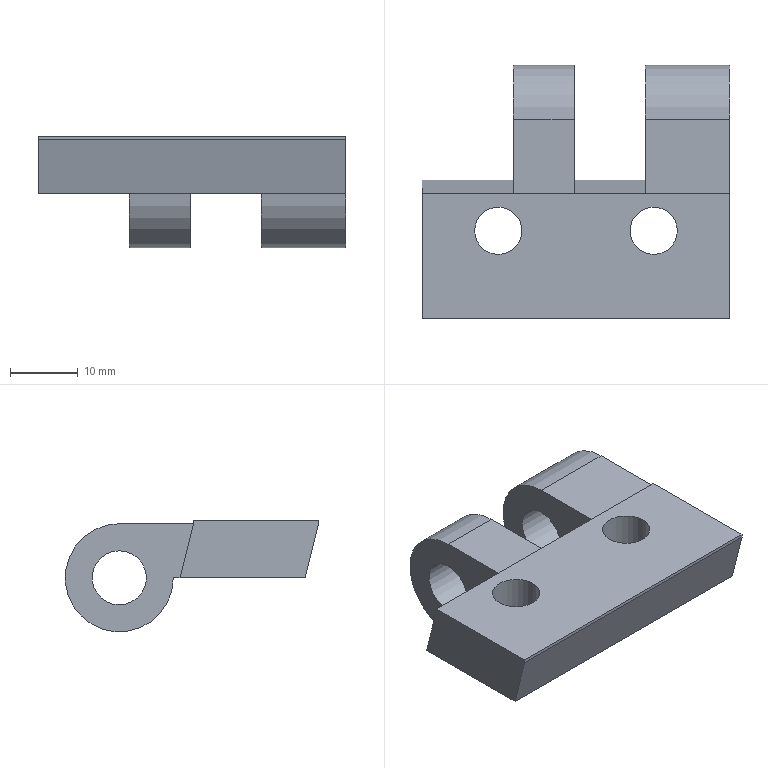Part | NX | 1 solid | 22 faces | box 45.5 x 37.5 x 16.5 mm | volume 10172 mm3 | plane 14 | cylinder 6 | cone 2 | commonest cylinder face diameters 7 x2 8 x2 16 x2
STEP:
#1=CARTESIAN_POINT('',(5.5,-8.5,-8.));
#2=VERTEX_POINT('',#1);
#3=CARTESIAN_POINT('',(11.75,-8.5,-8.));
#4=DIRECTION('',(0.,0.,-1.));
#5=DIRECTION('',(-1.,0.,0.));
#6=AXIS2_PLACEMENT_3D('',#3,#4,#5);
#7=CIRCLE('',#6,6.25);
#8=EDGE_CURVE('',#2,#2,#7,.T.);
#9=ORIENTED_EDGE('',*,*,#8,.F.);
#10=EDGE_LOOP('',(#9));
#11=FACE_BOUND('',#10,.T.);
#12=CARTESIAN_POINT('',(10.5,-1.,-8.));
#13=VERTEX_POINT('',#12);
#14=CARTESIAN_POINT('',(0.,-1.,-8.));
#15=VERTEX_POINT('',#14);
#16=CARTESIAN_POINT('',(10.5,-1.,-8.));
#17=DIRECTION('',(-1.,0.,0.));
#18=VECTOR('',#17,1000.);
#19=LINE('',#16,#18);
#20=EDGE_CURVE('',#13,#15,#19,.T.);
#21=ORIENTED_EDGE('',*,*,#20,.F.);
#22=CARTESIAN_POINT('',(10.5,0.,-8.));
#23=VERTEX_POINT('',#22);
#24=CARTESIAN_POINT('',(10.5,-1.,-8.));
#25=DIRECTION('',(0.,1.,0.));
#26=VECTOR('',#25,1000.);
#27=LINE('',#24,#26);
#28=EDGE_CURVE('',#13,#23,#27,.T.);
#29=ORIENTED_EDGE('',*,*,#28,.T.);
#30=CARTESIAN_POINT('',(23.,0.,-8.));
#31=VERTEX_POINT('',#30);
#32=CARTESIAN_POINT('',(10.5,0.,-8.));
#33=DIRECTION('',(1.,0.,0.));
#34=VECTOR('',#33,1000.);
#35=LINE('',#32,#34);
#36=EDGE_CURVE('',#23,#31,#35,.T.);
#37=ORIENTED_EDGE('',*,*,#36,.T.);
#38=CARTESIAN_POINT('',(23.,-19.5,-8.));
#39=VERTEX_POINT('',#38);
#40=CARTESIAN_POINT('',(23.,-21.5,-8.));
#41=DIRECTION('',(0.,1.,0.));
#42=VECTOR('',#41,1000.);
#43=LINE('',#40,#42);
#44=EDGE_CURVE('',#39,#31,#43,.T.);
#45=ORIENTED_EDGE('',*,*,#44,.F.);
#46=CARTESIAN_POINT('',(-22.5,-19.5,-8.));
#47=VERTEX_POINT('',#46);
#48=CARTESIAN_POINT('',(0.,-19.5,-8.));
#49=DIRECTION('',(-1.,0.,0.));
#50=VECTOR('',#49,1000.);
#51=LINE('',#48,#50);
#52=EDGE_CURVE('',#47,#39,#51,.F.);
#53=ORIENTED_EDGE('',*,*,#52,.F.);
#54=CARTESIAN_POINT('',(-22.5,-1.,-8.));
#55=VERTEX_POINT('',#54);
#56=CARTESIAN_POINT('',(-22.5,-21.5,-8.));
#57=DIRECTION('',(0.,-1.,0.));
#58=VECTOR('',#57,1000.);
#59=LINE('',#56,#58);
#60=EDGE_CURVE('',#55,#47,#59,.T.);
#61=ORIENTED_EDGE('',*,*,#60,.F.);
#62=CARTESIAN_POINT('',(-9.,-1.,-8.));
#63=VERTEX_POINT('',#62);
#64=CARTESIAN_POINT('',(-22.5,-1.,-8.));
#65=DIRECTION('',(1.,0.,0.));
#66=VECTOR('',#65,1000.);
#67=LINE('',#64,#66);
#68=EDGE_CURVE('',#55,#63,#67,.T.);
#69=ORIENTED_EDGE('',*,*,#68,.T.);
#70=CARTESIAN_POINT('',(-9.,0.,-8.));
#71=VERTEX_POINT('',#70);
#72=CARTESIAN_POINT('',(-9.,-21.5,-8.));
#73=DIRECTION('',(0.,-1.,0.));
#74=VECTOR('',#73,1000.);
#75=LINE('',#72,#74);
#76=EDGE_CURVE('',#71,#63,#75,.T.);
#77=ORIENTED_EDGE('',*,*,#76,.F.);
#78=CARTESIAN_POINT('',(0.,0.,-8.));
#79=VERTEX_POINT('',#78);
#80=CARTESIAN_POINT('',(-9.,0.,-8.));
#81=DIRECTION('',(1.,0.,0.));
#82=VECTOR('',#81,1000.);
#83=LINE('',#80,#82);
#84=EDGE_CURVE('',#71,#79,#83,.T.);
#85=ORIENTED_EDGE('',*,*,#84,.T.);
#86=CARTESIAN_POINT('',(0.,-21.5,-8.));
#87=DIRECTION('',(0.,-1.,0.));
#88=VECTOR('',#87,1000.);
#89=LINE('',#86,#88);
#90=EDGE_CURVE('',#79,#15,#89,.T.);
#91=ORIENTED_EDGE('',*,*,#90,.T.);
#92=EDGE_LOOP('',(#21,#29,#37,#45,#53,#61,#69,#77,#85,#91));
#93=FACE_BOUND('',#92,.T.);
#94=CARTESIAN_POINT('',(-17.5,-8.5,-8.));
#95=VERTEX_POINT('',#94);
#96=CARTESIAN_POINT('',(-11.25,-8.5,-8.));
#97=DIRECTION('',(0.,0.,-1.));
#98=DIRECTION('',(-1.,0.,0.));
#99=AXIS2_PLACEMENT_3D('',#96,#97,#98);
#100=CIRCLE('',#99,6.25);
#101=EDGE_CURVE('',#95,#95,#100,.T.);
#102=ORIENTED_EDGE('',*,*,#101,.F.);
#103=EDGE_LOOP('',(#102));
#104=FACE_BOUND('',#103,.T.);
#105=CARTESIAN_POINT('',(23.,-21.5,-8.));
#106=DIRECTION('',(0.,0.,1.));
#107=DIRECTION('',(1.,0.,0.));
#108=AXIS2_PLACEMENT_3D('',#105,#106,#107);
#109=PLANE('',#108);
#110=ADVANCED_FACE('',(#11,#93,#104),#109,.F.);
#111=CARTESIAN_POINT('',(-9.,-3.,0.));
#112=VERTEX_POINT('',#111);
#113=CARTESIAN_POINT('',(-9.,8.,0.));
#114=VERTEX_POINT('',#113);
#115=CARTESIAN_POINT('',(-9.,8.,0.));
#116=DIRECTION('',(0.,1.,0.));
#117=VECTOR('',#116,1000.);
#118=LINE('',#115,#117);
#119=EDGE_CURVE('',#112,#114,#118,.T.);
#120=ORIENTED_EDGE('',*,*,#119,.F.);
#121=CARTESIAN_POINT('',(0.,-3.,0.));
#122=VERTEX_POINT('',#121);
#123=CARTESIAN_POINT('',(-22.5,-3.,0.));
#124=DIRECTION('',(-1.,0.,0.));
#125=VECTOR('',#124,1000.);
#126=LINE('',#123,#125);
#127=EDGE_CURVE('',#122,#112,#126,.T.);
#128=ORIENTED_EDGE('',*,*,#127,.F.);
#129=CARTESIAN_POINT('',(0.,8.,0.));
#130=VERTEX_POINT('',#129);
#131=CARTESIAN_POINT('',(0.,8.,0.));
#132=DIRECTION('',(0.,1.,0.));
#133=VECTOR('',#132,1000.);
#134=LINE('',#131,#133);
#135=EDGE_CURVE('',#122,#130,#134,.T.);
#136=ORIENTED_EDGE('',*,*,#135,.T.);
#137=CARTESIAN_POINT('',(-9.,8.,0.));
#138=DIRECTION('',(1.,0.,0.));
#139=VECTOR('',#138,1000.);
#140=LINE('',#137,#139);
#141=EDGE_CURVE('',#114,#130,#140,.T.);
#142=ORIENTED_EDGE('',*,*,#141,.F.);
#143=EDGE_LOOP('',(#120,#128,#136,#142));
#144=FACE_BOUND('',#143,.T.);
#145=CARTESIAN_POINT('',(10.5,8.,0.));
#146=DIRECTION('',(0.,0.,1.));
#147=DIRECTION('',(1.,0.,0.));
#148=AXIS2_PLACEMENT_3D('',#145,#146,#147);
#149=PLANE('',#148);
#150=ADVANCED_FACE('',(#144),#149,.T.);
#151=CARTESIAN_POINT('',(10.5,8.,0.));
#152=VERTEX_POINT('',#151);
#153=CARTESIAN_POINT('',(10.5,-3.,0.));
#154=VERTEX_POINT('',#153);
#155=CARTESIAN_POINT('',(10.5,8.,0.));
#156=DIRECTION('',(0.,-1.,0.));
#157=VECTOR('',#156,1000.);
#158=LINE('',#155,#157);
#159=EDGE_CURVE('',#152,#154,#158,.T.);
#160=ORIENTED_EDGE('',*,*,#159,.T.);
#161=CARTESIAN_POINT('',(23.,-3.,0.));
#162=VERTEX_POINT('',#161);
#163=CARTESIAN_POINT('',(-22.5,-3.,0.));
#164=DIRECTION('',(-1.,0.,0.));
#165=VECTOR('',#164,1000.);
#166=LINE('',#163,#165);
#167=EDGE_CURVE('',#162,#154,#166,.T.);
#168=ORIENTED_EDGE('',*,*,#167,.F.);
#169=CARTESIAN_POINT('',(23.,8.,0.));
#170=VERTEX_POINT('',#169);
#171=CARTESIAN_POINT('',(23.,8.,0.));
#172=DIRECTION('',(0.,-1.,0.));
#173=VECTOR('',#172,1000.);
#174=LINE('',#171,#173);
#175=EDGE_CURVE('',#170,#162,#174,.T.);
#176=ORIENTED_EDGE('',*,*,#175,.F.);
#177=CARTESIAN_POINT('',(10.5,8.,0.));
#178=DIRECTION('',(1.,0.,0.));
#179=VECTOR('',#178,1000.);
#180=LINE('',#177,#179);
#181=EDGE_CURVE('',#152,#170,#180,.T.);
#182=ORIENTED_EDGE('',*,*,#181,.F.);
#183=EDGE_LOOP('',(#160,#168,#176,#182));
#184=FACE_BOUND('',#183,.T.);
#185=CARTESIAN_POINT('',(10.5,8.,0.));
#186=DIRECTION('',(0.,0.,1.));
#187=DIRECTION('',(1.,0.,0.));
#188=AXIS2_PLACEMENT_3D('',#185,#186,#187);
#189=PLANE('',#188);
#190=ADVANCED_FACE('',(#184),#189,.T.);
#191=CARTESIAN_POINT('',(-9.,8.,-12.));
#192=VERTEX_POINT('',#191);
#193=CARTESIAN_POINT('',(-9.,8.,-8.));
#194=DIRECTION('',(1.,0.,0.));
#195=DIRECTION('',(0.,0.,-1.));
#196=AXIS2_PLACEMENT_3D('',#193,#194,#195);
#197=CIRCLE('',#196,4.);
#198=EDGE_CURVE('',#192,#192,#197,.T.);
#199=ORIENTED_EDGE('',*,*,#198,.T.);
#200=EDGE_LOOP('',(#199));
#201=FACE_BOUND('',#200,.T.);
#202=CARTESIAN_POINT('',(-9.,-0.4706,-10.118));
#203=DIRECTION('',(0.,-0.2425,0.9701));
#204=VECTOR('',#203,1000.);
#205=LINE('',#202,#204);
#206=EDGE_CURVE('',#112,#63,#205,.F.);
#207=ORIENTED_EDGE('',*,*,#206,.F.);
#208=ORIENTED_EDGE('',*,*,#119,.T.);
#209=CARTESIAN_POINT('',(-9.,8.,-8.));
#210=DIRECTION('',(-1.,0.,0.));
#211=DIRECTION('',(0.,0.,-1.));
#212=AXIS2_PLACEMENT_3D('',#209,#210,#211);
#213=CIRCLE('',#212,8.);
#214=EDGE_CURVE('',#114,#71,#213,.T.);
#215=ORIENTED_EDGE('',*,*,#214,.T.);
#216=ORIENTED_EDGE('',*,*,#76,.T.);
#217=EDGE_LOOP('',(#207,#208,#215,#216));
#218=FACE_BOUND('',#217,.T.);
#219=CARTESIAN_POINT('',(-9.,8.,-8.));
#220=DIRECTION('',(1.,0.,0.));
#221=DIRECTION('',(0.,0.,-1.));
#222=AXIS2_PLACEMENT_3D('',#219,#220,#221);
#223=PLANE('',#222);
#224=ADVANCED_FACE('',(#201,#218),#223,.F.);
#225=CARTESIAN_POINT('',(23.,8.,-8.));
#226=DIRECTION('',(1.,0.,0.));
#227=DIRECTION('',(0.,0.,-1.));
#228=AXIS2_PLACEMENT_3D('',#225,#226,#227);
#229=CIRCLE('',#228,8.);
#230=EDGE_CURVE('',#31,#170,#229,.T.);
#231=ORIENTED_EDGE('',*,*,#230,.F.);
#232=ORIENTED_EDGE('',*,*,#36,.F.);
#233=CARTESIAN_POINT('',(10.5,8.,-8.));
#234=DIRECTION('',(1.,0.,0.));
#235=DIRECTION('',(0.,0.,-1.));
#236=AXIS2_PLACEMENT_3D('',#233,#234,#235);
#237=CIRCLE('',#236,8.);
#238=EDGE_CURVE('',#23,#152,#237,.T.);
#239=ORIENTED_EDGE('',*,*,#238,.T.);
#240=ORIENTED_EDGE('',*,*,#181,.T.);
#241=EDGE_LOOP('',(#231,#232,#239,#240));
#242=FACE_BOUND('',#241,.T.);
#243=CARTESIAN_POINT('',(10.5,8.,-8.));
#244=DIRECTION('',(1.,0.,0.));
#245=DIRECTION('',(0.,0.,-1.));
#246=AXIS2_PLACEMENT_3D('',#243,#244,#245);
#247=CYLINDRICAL_SURFACE('',#246,8.);
#248=ADVANCED_FACE('',(#242),#247,.T.);
#249=CARTESIAN_POINT('',(10.5,8.,-12.));
#250=VERTEX_POINT('',#249);
#251=CARTESIAN_POINT('',(10.5,8.,-8.));
#252=DIRECTION('',(1.,0.,0.));
#253=DIRECTION('',(0.,0.,-1.));
#254=AXIS2_PLACEMENT_3D('',#251,#252,#253);
#255=CIRCLE('',#254,4.);
#256=EDGE_CURVE('',#250,#250,#255,.T.);
#257=ORIENTED_EDGE('',*,*,#256,.T.);
#258=EDGE_LOOP('',(#257));
#259=FACE_BOUND('',#258,.T.);
#260=ORIENTED_EDGE('',*,*,#238,.F.);
#261=ORIENTED_EDGE('',*,*,#28,.F.);
#262=CARTESIAN_POINT('',(10.5,-1.,-8.));
#263=DIRECTION('',(0.,0.2425,-0.9701));
#264=VECTOR('',#263,1000.);
#265=LINE('',#262,#264);
#266=EDGE_CURVE('',#154,#13,#265,.T.);
#267=ORIENTED_EDGE('',*,*,#266,.F.);
#268=ORIENTED_EDGE('',*,*,#159,.F.);
#269=EDGE_LOOP('',(#260,#261,#267,#268));
#270=FACE_BOUND('',#269,.T.);
#271=CARTESIAN_POINT('',(10.5,8.,-8.));
#272=DIRECTION('',(1.,0.,0.));
#273=DIRECTION('',(0.,0.,-1.));
#274=AXIS2_PLACEMENT_3D('',#271,#272,#273);
#275=PLANE('',#274);
#276=ADVANCED_FACE('',(#259,#270),#275,.F.);
#277=CARTESIAN_POINT('',(23.,8.,-12.));
#278=VERTEX_POINT('',#277);
#279=CARTESIAN_POINT('',(23.,8.,-8.));
#280=DIRECTION('',(1.,0.,0.));
#281=DIRECTION('',(0.,0.,-1.));
#282=AXIS2_PLACEMENT_3D('',#279,#280,#281);
#283=CIRCLE('',#282,4.);
#284=EDGE_CURVE('',#278,#278,#283,.T.);
#285=ORIENTED_EDGE('',*,*,#284,.F.);
#286=EDGE_LOOP('',(#285));
#287=FACE_BOUND('',#286,.T.);
#288=ORIENTED_EDGE('',*,*,#230,.T.);
#289=ORIENTED_EDGE('',*,*,#175,.T.);
#290=CARTESIAN_POINT('',(23.,-3.,0.5));
#291=VERTEX_POINT('',#290);
#292=CARTESIAN_POINT('',(23.,-3.,0.5));
#293=DIRECTION('',(0.,0.,-1.));
#294=VECTOR('',#293,1000.);
#295=LINE('',#292,#294);
#296=EDGE_CURVE('',#291,#162,#295,.T.);
#297=ORIENTED_EDGE('',*,*,#296,.F.);
#298=CARTESIAN_POINT('',(23.,-21.5,0.5));
#299=VERTEX_POINT('',#298);
#300=CARTESIAN_POINT('',(23.,-3.,0.5));
#301=DIRECTION('',(0.,1.,0.));
#302=VECTOR('',#301,1000.);
#303=LINE('',#300,#302);
#304=EDGE_CURVE('',#299,#291,#303,.T.);
#305=ORIENTED_EDGE('',*,*,#304,.F.);
#306=CARTESIAN_POINT('',(23.,-21.5,0.));
#307=VERTEX_POINT('',#306);
#308=CARTESIAN_POINT('',(23.,-21.5,0.5));
#309=DIRECTION('',(0.,0.,-1.));
#310=VECTOR('',#309,1000.);
#311=LINE('',#308,#310);
#312=EDGE_CURVE('',#299,#307,#311,.T.);
#313=ORIENTED_EDGE('',*,*,#312,.T.);
#314=CARTESIAN_POINT('',(23.,-17.882,-14.471));
#315=DIRECTION('',(0.,0.2425,-0.9701));
#316=VECTOR('',#315,1000.);
#317=LINE('',#314,#316);
#318=EDGE_CURVE('',#39,#307,#317,.F.);
#319=ORIENTED_EDGE('',*,*,#318,.F.);
#320=ORIENTED_EDGE('',*,*,#44,.T.);
#321=EDGE_LOOP('',(#288,#289,#297,#305,#313,#319,#320));
#322=FACE_BOUND('',#321,.T.);
#323=CARTESIAN_POINT('',(23.,8.,-8.));
#324=DIRECTION('',(1.,0.,0.));
#325=DIRECTION('',(0.,0.,-1.));
#326=AXIS2_PLACEMENT_3D('',#323,#324,#325);
#327=PLANE('',#326);
#328=ADVANCED_FACE('',(#287,#322),#327,.T.);
#329=CARTESIAN_POINT('',(-22.5,-21.5,0.));
#330=VERTEX_POINT('',#329);
#331=CARTESIAN_POINT('',(0.,-21.5,0.));
#332=DIRECTION('',(-1.,0.,0.));
#333=VECTOR('',#332,1000.);
#334=LINE('',#331,#333);
#335=EDGE_CURVE('',#307,#330,#334,.T.);
#336=ORIENTED_EDGE('',*,*,#335,.T.);
#337=CARTESIAN_POINT('',(-22.5,-20.235,-5.059));
#338=DIRECTION('',(0.,0.2425,-0.9701));
#339=VECTOR('',#338,1000.);
#340=LINE('',#337,#339);
#341=EDGE_CURVE('',#47,#330,#340,.F.);
#342=ORIENTED_EDGE('',*,*,#341,.F.);
#343=ORIENTED_EDGE('',*,*,#52,.T.);
#344=ORIENTED_EDGE('',*,*,#318,.T.);
#345=EDGE_LOOP('',(#336,#342,#343,#344));
#346=FACE_BOUND('',#345,.T.);
#347=CARTESIAN_POINT('',(0.,-21.5,0.));
#348=DIRECTION('',(0.,-0.9701,-0.2425));
#349=DIRECTION('',(0.,0.2425,-0.9701));
#350=AXIS2_PLACEMENT_3D('',#347,#348,#349);
#351=PLANE('',#350);
#352=ADVANCED_FACE('',(#346),#351,.T.);
#353=ORIENTED_EDGE('',*,*,#266,.T.);
#354=ORIENTED_EDGE('',*,*,#20,.T.);
#355=CARTESIAN_POINT('',(0.,-0.4706,-10.118));
#356=DIRECTION('',(0.,-0.2425,0.9701));
#357=VECTOR('',#356,1000.);
#358=LINE('',#355,#357);
#359=EDGE_CURVE('',#15,#122,#358,.T.);
#360=ORIENTED_EDGE('',*,*,#359,.T.);
#361=CARTESIAN_POINT('',(10.5,-3.,0.));
#362=DIRECTION('',(1.,0.,0.));
#363=VECTOR('',#362,1000.);
#364=LINE('',#361,#363);
#365=EDGE_CURVE('',#122,#154,#364,.T.);
#366=ORIENTED_EDGE('',*,*,#365,.T.);
#367=EDGE_LOOP('',(#353,#354,#360,#366));
#368=FACE_BOUND('',#367,.T.);
#369=CARTESIAN_POINT('',(10.5,-1.,-8.));
#370=DIRECTION('',(0.,0.9701,0.2425));
#371=DIRECTION('',(0.,-0.2425,0.9701));
#372=AXIS2_PLACEMENT_3D('',#369,#370,#371);
#373=PLANE('',#372);
#374=ADVANCED_FACE('',(#368),#373,.T.);
#375=CARTESIAN_POINT('',(0.,8.,-12.));
#376=VERTEX_POINT('',#375);
#377=CARTESIAN_POINT('',(0.,8.,-8.));
#378=DIRECTION('',(1.,0.,0.));
#379=DIRECTION('',(0.,0.,-1.));
#380=AXIS2_PLACEMENT_3D('',#377,#378,#379);
#381=CIRCLE('',#380,4.);
#382=EDGE_CURVE('',#376,#376,#381,.T.);
#383=ORIENTED_EDGE('',*,*,#382,.F.);
#384=EDGE_LOOP('',(#383));
#385=FACE_BOUND('',#384,.T.);
#386=ORIENTED_EDGE('',*,*,#359,.F.);
#387=ORIENTED_EDGE('',*,*,#90,.F.);
#388=CARTESIAN_POINT('',(0.,8.,-8.));
#389=DIRECTION('',(-1.,0.,0.));
#390=DIRECTION('',(0.,0.,-1.));
#391=AXIS2_PLACEMENT_3D('',#388,#389,#390);
#392=CIRCLE('',#391,8.);
#393=EDGE_CURVE('',#130,#79,#392,.T.);
#394=ORIENTED_EDGE('',*,*,#393,.F.);
#395=ORIENTED_EDGE('',*,*,#135,.F.);
#396=EDGE_LOOP('',(#386,#387,#394,#395));
#397=FACE_BOUND('',#396,.T.);
#398=CARTESIAN_POINT('',(0.,8.,-8.));
#399=DIRECTION('',(1.,0.,0.));
#400=DIRECTION('',(0.,0.,-1.));
#401=AXIS2_PLACEMENT_3D('',#398,#399,#400);
#402=PLANE('',#401);
#403=ADVANCED_FACE('',(#385,#397),#402,.T.);
#404=ORIENTED_EDGE('',*,*,#393,.T.);
#405=ORIENTED_EDGE('',*,*,#84,.F.);
#406=ORIENTED_EDGE('',*,*,#214,.F.);
#407=ORIENTED_EDGE('',*,*,#141,.T.);
#408=EDGE_LOOP('',(#404,#405,#406,#407));
#409=FACE_BOUND('',#408,.T.);
#410=CARTESIAN_POINT('',(-9.,8.,-8.));
#411=DIRECTION('',(1.,0.,0.));
#412=DIRECTION('',(0.,0.,-1.));
#413=AXIS2_PLACEMENT_3D('',#410,#411,#412);
#414=CYLINDRICAL_SURFACE('',#413,8.);
#415=ADVANCED_FACE('',(#409),#414,.T.);
#416=ORIENTED_EDGE('',*,*,#206,.T.);
#417=ORIENTED_EDGE('',*,*,#68,.F.);
#418=CARTESIAN_POINT('',(-22.5,-3.,0.));
#419=VERTEX_POINT('',#418);
#420=CARTESIAN_POINT('',(-22.5,-2.824,-0.7059));
#421=DIRECTION('',(0.,-0.2425,0.9701));
#422=VECTOR('',#421,1000.);
#423=LINE('',#420,#422);
#424=EDGE_CURVE('',#419,#55,#423,.F.);
#425=ORIENTED_EDGE('',*,*,#424,.F.);
#426=CARTESIAN_POINT('',(10.5,-3.,0.));
#427=DIRECTION('',(-1.,0.,0.));
#428=VECTOR('',#427,1000.);
#429=LINE('',#426,#428);
#430=EDGE_CURVE('',#419,#112,#429,.F.);
#431=ORIENTED_EDGE('',*,*,#430,.T.);
#432=EDGE_LOOP('',(#416,#417,#425,#431));
#433=FACE_BOUND('',#432,.T.);
#434=CARTESIAN_POINT('',(-22.5,-1.,-8.));
#435=DIRECTION('',(0.,0.9701,0.2425));
#436=DIRECTION('',(0.,-0.2425,0.9701));
#437=AXIS2_PLACEMENT_3D('',#434,#435,#436);
#438=PLANE('',#437);
#439=ADVANCED_FACE('',(#433),#438,.T.);
#440=ORIENTED_EDGE('',*,*,#341,.T.);
#441=CARTESIAN_POINT('',(-22.5,-21.5,0.5));
#442=VERTEX_POINT('',#441);
#443=CARTESIAN_POINT('',(-22.5,-21.5,0.5));
#444=DIRECTION('',(0.,0.,-1.));
#445=VECTOR('',#444,1000.);
#446=LINE('',#443,#445);
#447=EDGE_CURVE('',#442,#330,#446,.T.);
#448=ORIENTED_EDGE('',*,*,#447,.F.);
#449=CARTESIAN_POINT('',(-22.5,-3.,0.5));
#450=VERTEX_POINT('',#449);
#451=CARTESIAN_POINT('',(-22.5,-3.,0.5));
#452=DIRECTION('',(0.,-1.,0.));
#453=VECTOR('',#452,1000.);
#454=LINE('',#451,#453);
#455=EDGE_CURVE('',#450,#442,#454,.T.);
#456=ORIENTED_EDGE('',*,*,#455,.F.);
#457=CARTESIAN_POINT('',(-22.5,-3.,0.5));
#458=DIRECTION('',(0.,0.,-1.));
#459=VECTOR('',#458,1000.);
#460=LINE('',#457,#459);
#461=EDGE_CURVE('',#450,#419,#460,.T.);
#462=ORIENTED_EDGE('',*,*,#461,.T.);
#463=ORIENTED_EDGE('',*,*,#424,.T.);
#464=ORIENTED_EDGE('',*,*,#60,.T.);
#465=EDGE_LOOP('',(#440,#448,#456,#462,#463,#464));
#466=FACE_BOUND('',#465,.T.);
#467=CARTESIAN_POINT('',(-22.5,0.,0.));
#468=DIRECTION('',(1.,0.,0.));
#469=DIRECTION('',(0.,0.,-1.));
#470=AXIS2_PLACEMENT_3D('',#467,#468,#469);
#471=PLANE('',#470);
#472=ADVANCED_FACE('',(#466),#471,.F.);
#473=ORIENTED_EDGE('',*,*,#382,.T.);
#474=EDGE_LOOP('',(#473));
#475=FACE_BOUND('',#474,.T.);
#476=ORIENTED_EDGE('',*,*,#198,.F.);
#477=EDGE_LOOP('',(#476));
#478=FACE_BOUND('',#477,.T.);
#479=CARTESIAN_POINT('',(-17.,8.,-8.));
#480=DIRECTION('',(1.,0.,0.));
#481=DIRECTION('',(0.,0.,-1.));
#482=AXIS2_PLACEMENT_3D('',#479,#480,#481);
#483=CYLINDRICAL_SURFACE('',#482,4.);
#484=ADVANCED_FACE('',(#475,#478),#483,.F.);
#485=ORIENTED_EDGE('',*,*,#284,.T.);
#486=EDGE_LOOP('',(#485));
#487=FACE_BOUND('',#486,.T.);
#488=ORIENTED_EDGE('',*,*,#256,.F.);
#489=EDGE_LOOP('',(#488));
#490=FACE_BOUND('',#489,.T.);
#491=CARTESIAN_POINT('',(-17.,8.,-8.));
#492=DIRECTION('',(1.,0.,0.));
#493=DIRECTION('',(0.,0.,-1.));
#494=AXIS2_PLACEMENT_3D('',#491,#492,#493);
#495=CYLINDRICAL_SURFACE('',#494,4.);
#496=ADVANCED_FACE('',(#487,#490),#495,.F.);
#497=ORIENTED_EDGE('',*,*,#335,.F.);
#498=ORIENTED_EDGE('',*,*,#312,.F.);
#499=CARTESIAN_POINT('',(-22.5,-21.5,0.5));
#500=DIRECTION('',(1.,0.,0.));
#501=VECTOR('',#500,1000.);
#502=LINE('',#499,#501);
#503=EDGE_CURVE('',#442,#299,#502,.T.);
#504=ORIENTED_EDGE('',*,*,#503,.F.);
#505=ORIENTED_EDGE('',*,*,#447,.T.);
#506=EDGE_LOOP('',(#497,#498,#504,#505));
#507=FACE_BOUND('',#506,.T.);
#508=CARTESIAN_POINT('',(-22.5,-21.5,0.5));
#509=DIRECTION('',(0.,1.,0.));
#510=DIRECTION('',(0.,0.,1.));
#511=AXIS2_PLACEMENT_3D('',#508,#509,#510);
#512=PLANE('',#511);
#513=ADVANCED_FACE('',(#507),#512,.F.);
#514=ORIENTED_EDGE('',*,*,#167,.T.);
#515=ORIENTED_EDGE('',*,*,#365,.F.);
#516=ORIENTED_EDGE('',*,*,#127,.T.);
#517=ORIENTED_EDGE('',*,*,#430,.F.);
#518=ORIENTED_EDGE('',*,*,#461,.F.);
#519=CARTESIAN_POINT('',(-22.5,-3.,0.5));
#520=DIRECTION('',(-1.,0.,0.));
#521=VECTOR('',#520,1000.);
#522=LINE('',#519,#521);
#523=EDGE_CURVE('',#291,#450,#522,.T.);
#524=ORIENTED_EDGE('',*,*,#523,.F.);
#525=ORIENTED_EDGE('',*,*,#296,.T.);
#526=EDGE_LOOP('',(#514,#515,#516,#517,#518,#524,#525));
#527=FACE_BOUND('',#526,.T.);
#528=CARTESIAN_POINT('',(-22.5,-3.,0.5));
#529=DIRECTION('',(0.,-1.,0.));
#530=DIRECTION('',(0.,0.,-1.));
#531=AXIS2_PLACEMENT_3D('',#528,#529,#530);
#532=PLANE('',#531);
#533=ADVANCED_FACE('',(#527),#532,.F.);
#534=CARTESIAN_POINT('',(8.25,-8.5,0.5));
#535=VERTEX_POINT('',#534);
#536=CARTESIAN_POINT('',(11.75,-8.5,0.5));
#537=DIRECTION('',(0.,0.,-1.));
#538=DIRECTION('',(-1.,0.,0.));
#539=AXIS2_PLACEMENT_3D('',#536,#537,#538);
#540=CIRCLE('',#539,3.5);
#541=EDGE_CURVE('',#535,#535,#540,.T.);
#542=ORIENTED_EDGE('',*,*,#541,.T.);
#543=EDGE_LOOP('',(#542));
#544=FACE_BOUND('',#543,.T.);
#545=CARTESIAN_POINT('',(-14.75,-8.5,0.5));
#546=VERTEX_POINT('',#545);
#547=CARTESIAN_POINT('',(-11.25,-8.5,0.5));
#548=DIRECTION('',(0.,0.,-1.));
#549=DIRECTION('',(-1.,0.,0.));
#550=AXIS2_PLACEMENT_3D('',#547,#548,#549);
#551=CIRCLE('',#550,3.5);
#552=EDGE_CURVE('',#546,#546,#551,.T.);
#553=ORIENTED_EDGE('',*,*,#552,.T.);
#554=EDGE_LOOP('',(#553));
#555=FACE_BOUND('',#554,.T.);
#556=ORIENTED_EDGE('',*,*,#455,.T.);
#557=ORIENTED_EDGE('',*,*,#503,.T.);
#558=ORIENTED_EDGE('',*,*,#304,.T.);
#559=ORIENTED_EDGE('',*,*,#523,.T.);
#560=EDGE_LOOP('',(#556,#557,#558,#559));
#561=FACE_BOUND('',#560,.T.);
#562=CARTESIAN_POINT('',(0.,0.,0.5));
#563=DIRECTION('',(0.,0.,1.));
#564=DIRECTION('',(1.,0.,0.));
#565=AXIS2_PLACEMENT_3D('',#562,#563,#564);
#566=PLANE('',#565);
#567=ADVANCED_FACE('',(#544,#555,#561),#566,.T.);
#568=ORIENTED_EDGE('',*,*,#552,.F.);
#569=EDGE_LOOP('',(#568));
#570=FACE_BOUND('',#569,.T.);
#571=CARTESIAN_POINT('',(-14.75,-8.5,-5.25));
#572=VERTEX_POINT('',#571);
#573=CARTESIAN_POINT('',(-11.25,-8.5,-5.25));
#574=DIRECTION('',(0.,0.,-1.));
#575=DIRECTION('',(-1.,0.,0.));
#576=AXIS2_PLACEMENT_3D('',#573,#574,#575);
#577=CIRCLE('',#576,3.5);
#578=EDGE_CURVE('',#572,#572,#577,.T.);
#579=ORIENTED_EDGE('',*,*,#578,.T.);
#580=EDGE_LOOP('',(#579));
#581=FACE_BOUND('',#580,.T.);
#582=CARTESIAN_POINT('',(-11.25,-8.5,-8.));
#583=DIRECTION('',(0.,0.,-1.));
#584=DIRECTION('',(-1.,0.,0.));
#585=AXIS2_PLACEMENT_3D('',#582,#583,#584);
#586=CYLINDRICAL_SURFACE('',#585,3.5);
#587=ADVANCED_FACE('',(#570,#581),#586,.F.);
#588=ORIENTED_EDGE('',*,*,#578,.F.);
#589=EDGE_LOOP('',(#588));
#590=FACE_BOUND('',#589,.T.);
#591=ORIENTED_EDGE('',*,*,#101,.T.);
#592=EDGE_LOOP('',(#591));
#593=FACE_BOUND('',#592,.T.);
#594=CARTESIAN_POINT('',(-11.25,-8.5,-8.));
#595=DIRECTION('',(0.,0.,-1.));
#596=DIRECTION('',(-1.,0.,0.));
#597=AXIS2_PLACEMENT_3D('',#594,#595,#596);
#598=CONICAL_SURFACE('',#597,6.25,0.7854);
#599=ADVANCED_FACE('',(#590,#593),#598,.F.);
#600=ORIENTED_EDGE('',*,*,#541,.F.);
#601=EDGE_LOOP('',(#600));
#602=FACE_BOUND('',#601,.T.);
#603=CARTESIAN_POINT('',(8.25,-8.5,-5.25));
#604=VERTEX_POINT('',#603);
#605=CARTESIAN_POINT('',(11.75,-8.5,-5.25));
#606=DIRECTION('',(0.,0.,-1.));
#607=DIRECTION('',(-1.,0.,0.));
#608=AXIS2_PLACEMENT_3D('',#605,#606,#607);
#609=CIRCLE('',#608,3.5);
#610=EDGE_CURVE('',#604,#604,#609,.T.);
#611=ORIENTED_EDGE('',*,*,#610,.T.);
#612=EDGE_LOOP('',(#611));
#613=FACE_BOUND('',#612,.T.);
#614=CARTESIAN_POINT('',(11.75,-8.5,-8.));
#615=DIRECTION('',(0.,0.,-1.));
#616=DIRECTION('',(-1.,0.,0.));
#617=AXIS2_PLACEMENT_3D('',#614,#615,#616);
#618=CYLINDRICAL_SURFACE('',#617,3.5);
#619=ADVANCED_FACE('',(#602,#613),#618,.F.);
#620=ORIENTED_EDGE('',*,*,#610,.F.);
#621=EDGE_LOOP('',(#620));
#622=FACE_BOUND('',#621,.T.);
#623=ORIENTED_EDGE('',*,*,#8,.T.);
#624=EDGE_LOOP('',(#623));
#625=FACE_BOUND('',#624,.T.);
#626=CARTESIAN_POINT('',(11.75,-8.5,-8.));
#627=DIRECTION('',(0.,0.,-1.));
#628=DIRECTION('',(-1.,0.,0.));
#629=AXIS2_PLACEMENT_3D('',#626,#627,#628);
#630=CONICAL_SURFACE('',#629,6.25,0.7854);
#631=ADVANCED_FACE('',(#622,#625),#630,.F.);
#632=CLOSED_SHELL('',(#110,#150,#190,#224,#248,#276,#328,#352,#374,#403,#415,#439,#472,#484,#496,#513,#533,#567,#587,#599,#619,#631));
#633=MANIFOLD_SOLID_BREP('',#632);
#634=(LENGTH_UNIT()NAMED_UNIT(*)SI_UNIT(.MILLI.,.METRE.));
#635=UNCERTAINTY_MEASURE_WITH_UNIT(LENGTH_MEASURE(0.00001),#634,'','');
#636=(NAMED_UNIT(*)PLANE_ANGLE_UNIT()SI_UNIT($,.RADIAN.));
#637=(NAMED_UNIT(*)SI_UNIT($,.STERADIAN.)SOLID_ANGLE_UNIT());
#638=(GEOMETRIC_REPRESENTATION_CONTEXT(3)GLOBAL_UNCERTAINTY_ASSIGNED_CONTEXT((#635))GLOBAL_UNIT_ASSIGNED_CONTEXT((#634,#636,#637))REPRESENTATION_CONTEXT('',''));
#639=ADVANCED_BREP_SHAPE_REPRESENTATION('',(#633),#638);